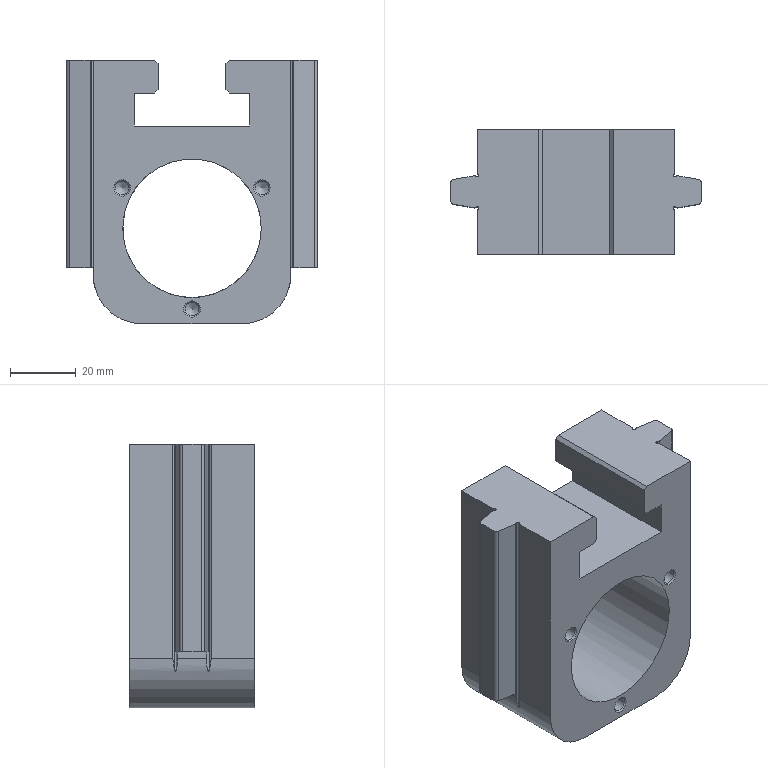Part | STEP file | YBQDJ-YB-7 | 1 solid | 70 faces | box 76 x 38 x 80 mm | volume 112101 mm3 | plane 30 | cylinder 26 | cone 14 | commonest cylinder face diameters 1 x12 4.2 x7 2 x4 30 x2 42 x1